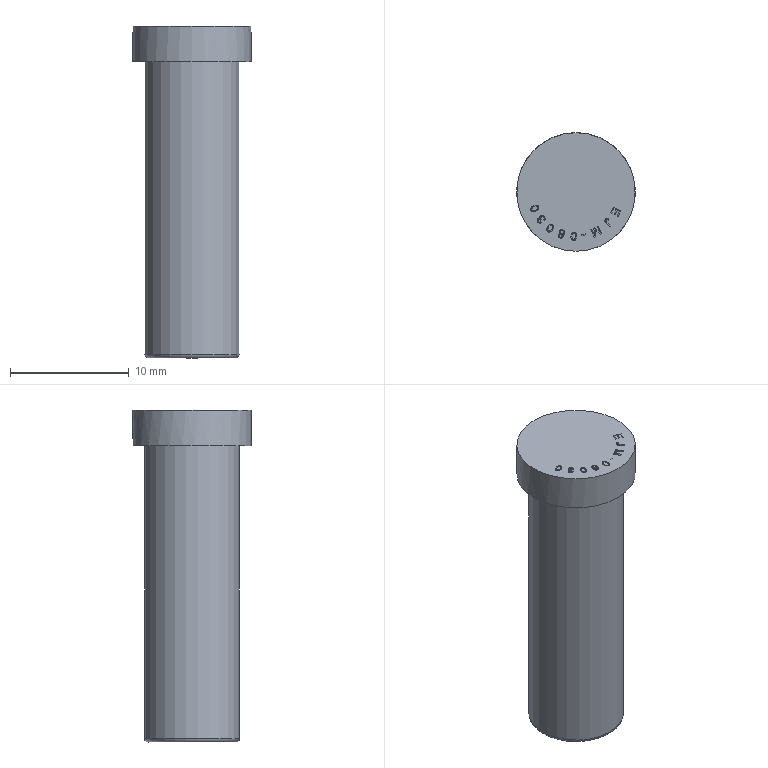Part | STEP file | lll_id3062_x_t | 1 solid | 82 faces | box 10 x 10 x 28 mm | volume 1492 mm3 | plane 49 | other 30 | cylinder 2 | torus 1 | commonest cylinder face diameters 8 x1 10 x1